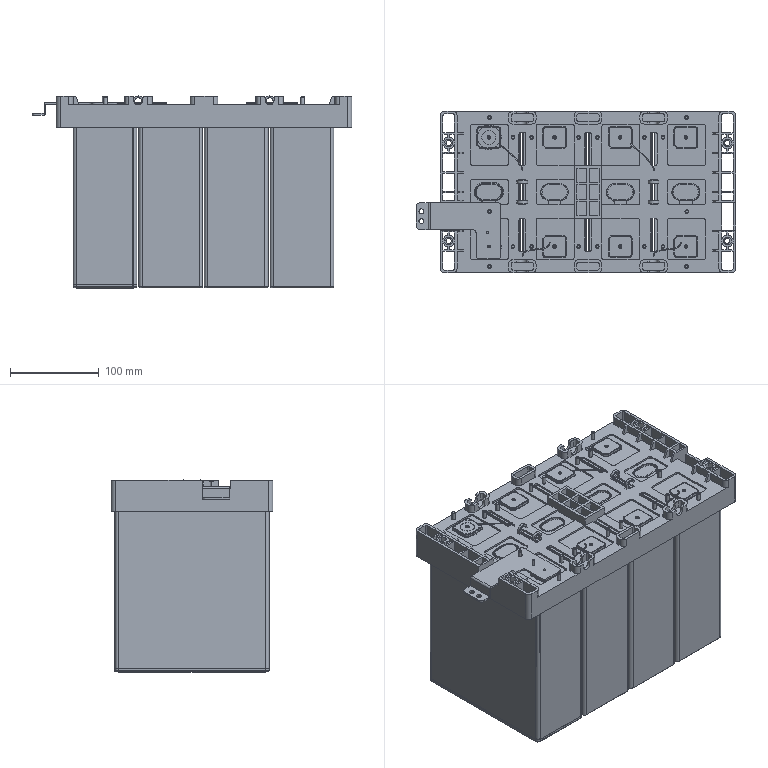Part | NX | features BREP 20 | 20 solids | 2669 faces | box 360 x 182 x 216.365 mm | volume 10554329 mm3 | plane 1529 | cylinder 910 | cone 112 | torus 74 | spline 40 | sphere 4 | commonest cylinder face diameters 6 x182 4 x136 3 x76 2 x60 10 x52 8 x46